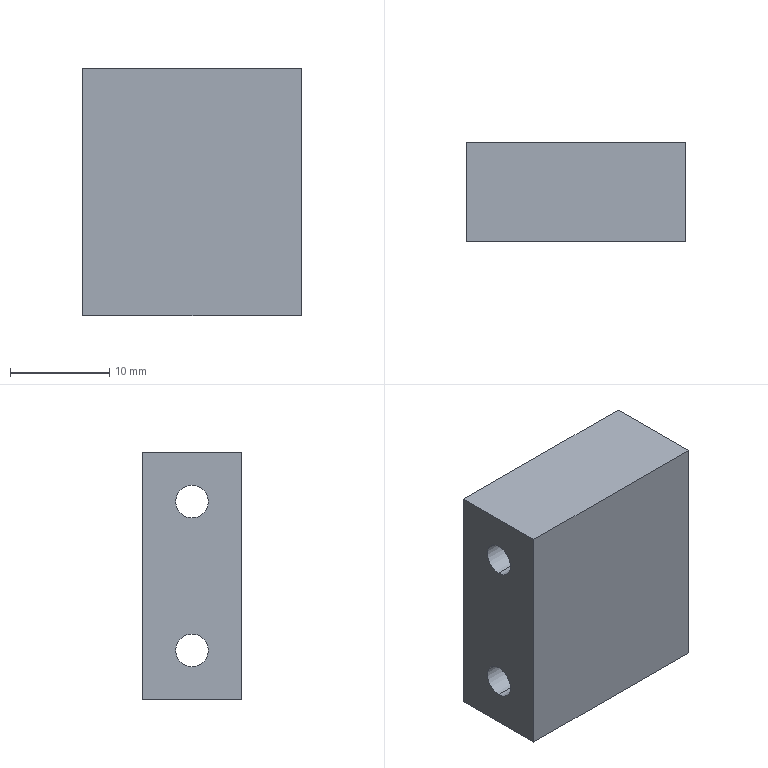Part | STEP file | 0246_220_Pin | 1 solid | 10 faces | box 22 x 10 x 25 mm | volume 5124 mm3 | plane 6 | cylinder 4 | commonest cylinder face diameters 3.3 x4
STEP:
#1=CARTESIAN_POINT('',(0.,0.,0.));
#2=DIRECTION('',(0.,0.,1.));
#3=DIRECTION('',(1.,0.,0.));
#4=AXIS2_PLACEMENT_3D('',#1,#2,#3);
#5=CARTESIAN_POINT('',(0.,5.,-5.85));
#6=VERTEX_POINT('',#5);
#7=CARTESIAN_POINT('',(-22.,5.,-5.85));
#8=VERTEX_POINT('',#7);
#9=CARTESIAN_POINT('',(-22.,5.,-5.85));
#10=DIRECTION('',(-1.,0.,0.));
#11=VECTOR('',#10,1.);
#12=LINE('',#9,#11);
#13=CARTESIAN_POINT('',(-22.,5.,-7.5));
#14=DIRECTION('',(-1.,0.,0.));
#15=DIRECTION('',(0.,0.,1.));
#16=AXIS2_PLACEMENT_3D('',#13,#14,#15);
#17=CYLINDRICAL_SURFACE('',#16,1.65);
#18=CARTESIAN_POINT('',(6.283,0.));
#19=DIRECTION('',(0.,1.));
#20=VECTOR('',#19,1.);
#21=LINE('',#18,#20);
#22=(GEOMETRIC_REPRESENTATION_CONTEXT(2)PARAMETRIC_REPRESENTATION_CONTEXT()REPRESENTATION_CONTEXT('',''));
#23=DEFINITIONAL_REPRESENTATION('',(#21),#22);
#24=PCURVE('',#17,#23);
#25=CARTESIAN_POINT('',(-22.,5.,-7.5));
#26=DIRECTION('',(-1.,0.,0.));
#27=DIRECTION('',(0.,0.,1.));
#28=AXIS2_PLACEMENT_3D('',#25,#26,#27);
#29=CYLINDRICAL_SURFACE('',#28,1.65);
#30=CARTESIAN_POINT('',(0.,0.));
#31=DIRECTION('',(0.,1.));
#32=VECTOR('',#31,1.);
#33=LINE('',#30,#32);
#34=(GEOMETRIC_REPRESENTATION_CONTEXT(2)PARAMETRIC_REPRESENTATION_CONTEXT()REPRESENTATION_CONTEXT('',''));
#35=DEFINITIONAL_REPRESENTATION('',(#33),#34);
#36=PCURVE('',#29,#35);
#37=SURFACE_CURVE('',#12,(#24,#36),.PCURVE_S1.);
#38=EDGE_CURVE('',#6,#8,#37,.T.);
#39=ORIENTED_EDGE('',*,*,#38,.T.);
#40=CARTESIAN_POINT('',(-22.,5.,-9.15));
#41=VERTEX_POINT('',#40);
#42=CARTESIAN_POINT('',(-22.,5.,-7.5));
#43=DIRECTION('',(-1.,0.,0.));
#44=DIRECTION('',(0.,0.,1.));
#45=AXIS2_PLACEMENT_3D('',#42,#43,#44);
#46=CIRCLE('',#45,1.65);
#47=CARTESIAN_POINT('',(0.,0.));
#48=DIRECTION('',(1.,0.));
#49=VECTOR('',#48,1.);
#50=LINE('',#47,#49);
#51=(GEOMETRIC_REPRESENTATION_CONTEXT(2)PARAMETRIC_REPRESENTATION_CONTEXT()REPRESENTATION_CONTEXT('',''));
#52=DEFINITIONAL_REPRESENTATION('',(#50),#51);
#53=PCURVE('',#17,#52);
#54=CARTESIAN_POINT('',(-22.,10.,-12.5));
#55=DIRECTION('',(1.,0.,0.));
#56=DIRECTION('',(0.,0.,-1.));
#57=AXIS2_PLACEMENT_3D('',#54,#55,#56);
#58=PLANE('',#57);
#59=CARTESIAN_POINT('',(-6.65,-5.));
#60=CARTESIAN_POINT('',(-6.65,-2.142));
#61=CARTESIAN_POINT('',(-4.175,-3.571));
#62=CARTESIAN_POINT('',(-1.7,-5.));
#63=CARTESIAN_POINT('',(-4.175,-6.429));
#64=CARTESIAN_POINT('',(-6.65,-7.858));
#65=CARTESIAN_POINT('',(-6.65,-5.));
#66=(BOUNDED_CURVE()B_SPLINE_CURVE(2,(#59,#60,#61,#62,#63,#64,#65),.UNSPECIFIED.,.T.,.F.)B_SPLINE_CURVE_WITH_KNOTS((1,2,2,2,2,1),(-2.094,0.,2.094,4.189,6.283,8.378),.UNSPECIFIED.)CURVE()GEOMETRIC_REPRESENTATION_ITEM()RATIONAL_B_SPLINE_CURVE((1.,0.5,1.,0.5,1.,0.5,1.))REPRESENTATION_ITEM(''));
#67=(GEOMETRIC_REPRESENTATION_CONTEXT(2)PARAMETRIC_REPRESENTATION_CONTEXT()REPRESENTATION_CONTEXT('',''));
#68=DEFINITIONAL_REPRESENTATION('',(#66),#67);
#69=PCURVE('',#58,#68);
#70=SURFACE_CURVE('',#46,(#53,#69),.PCURVE_S1.);
#71=EDGE_CURVE('',#41,#8,#70,.T.);
#72=ORIENTED_EDGE('',*,*,#71,.F.);
#73=CARTESIAN_POINT('',(0.,5.,-9.15));
#74=VERTEX_POINT('',#73);
#75=CARTESIAN_POINT('',(-22.,5.,-9.15));
#76=DIRECTION('',(-1.,0.,0.));
#77=VECTOR('',#76,1.);
#78=LINE('',#75,#77);
#79=CARTESIAN_POINT('',(3.142,0.));
#80=DIRECTION('',(0.,1.));
#81=VECTOR('',#80,1.);
#82=LINE('',#79,#81);
#83=(GEOMETRIC_REPRESENTATION_CONTEXT(2)PARAMETRIC_REPRESENTATION_CONTEXT()REPRESENTATION_CONTEXT('',''));
#84=DEFINITIONAL_REPRESENTATION('',(#82),#83);
#85=PCURVE('',#17,#84);
#86=CARTESIAN_POINT('',(3.142,0.));
#87=DIRECTION('',(0.,1.));
#88=VECTOR('',#87,1.);
#89=LINE('',#86,#88);
#90=(GEOMETRIC_REPRESENTATION_CONTEXT(2)PARAMETRIC_REPRESENTATION_CONTEXT()REPRESENTATION_CONTEXT('',''));
#91=DEFINITIONAL_REPRESENTATION('',(#89),#90);
#92=PCURVE('',#29,#91);
#93=SURFACE_CURVE('',#78,(#85,#92),.PCURVE_S1.);
#94=EDGE_CURVE('',#74,#41,#93,.T.);
#95=ORIENTED_EDGE('',*,*,#94,.F.);
#96=CARTESIAN_POINT('',(0.,5.,-7.5));
#97=DIRECTION('',(-1.,0.,0.));
#98=DIRECTION('',(0.,0.,1.));
#99=AXIS2_PLACEMENT_3D('',#96,#97,#98);
#100=CIRCLE('',#99,1.65);
#101=CARTESIAN_POINT('',(0.,-22.));
#102=DIRECTION('',(1.,0.));
#103=VECTOR('',#102,1.);
#104=LINE('',#101,#103);
#105=(GEOMETRIC_REPRESENTATION_CONTEXT(2)PARAMETRIC_REPRESENTATION_CONTEXT()REPRESENTATION_CONTEXT('',''));
#106=DEFINITIONAL_REPRESENTATION('',(#104),#105);
#107=PCURVE('',#17,#106);
#108=CARTESIAN_POINT('',(0.,10.,-12.5));
#109=DIRECTION('',(-1.,0.,0.));
#110=DIRECTION('',(0.,0.,1.));
#111=AXIS2_PLACEMENT_3D('',#108,#109,#110);
#112=PLANE('',#111);
#113=CARTESIAN_POINT('',(5.,-5.));
#114=DIRECTION('',(1.,0.));
#115=AXIS2_PLACEMENT_2D('',#113,#114);
#116=CIRCLE('',#115,1.65);
#117=(GEOMETRIC_REPRESENTATION_CONTEXT(2)PARAMETRIC_REPRESENTATION_CONTEXT()REPRESENTATION_CONTEXT('',''));
#118=DEFINITIONAL_REPRESENTATION('',(#116),#117);
#119=PCURVE('',#112,#118);
#120=SURFACE_CURVE('',#100,(#107,#119),.PCURVE_S1.);
#121=EDGE_CURVE('',#74,#6,#120,.T.);
#122=ORIENTED_EDGE('',*,*,#121,.T.);
#123=EDGE_LOOP('',(#39,#72,#95,#122));
#124=FACE_BOUND('',#123,.F.);
#125=ADVANCED_FACE('',(#124),#17,.F.);
#126=CARTESIAN_POINT('',(0.,5.,9.15));
#127=VERTEX_POINT('',#126);
#128=CARTESIAN_POINT('',(-22.,5.,9.15));
#129=VERTEX_POINT('',#128);
#130=CARTESIAN_POINT('',(-22.,5.,9.15));
#131=DIRECTION('',(-1.,0.,0.));
#132=VECTOR('',#131,1.);
#133=LINE('',#130,#132);
#134=CARTESIAN_POINT('',(-22.,5.,7.5));
#135=DIRECTION('',(-1.,0.,0.));
#136=DIRECTION('',(0.,0.,1.));
#137=AXIS2_PLACEMENT_3D('',#134,#135,#136);
#138=CYLINDRICAL_SURFACE('',#137,1.65);
#139=CARTESIAN_POINT('',(6.283,0.));
#140=DIRECTION('',(0.,1.));
#141=VECTOR('',#140,1.);
#142=LINE('',#139,#141);
#143=(GEOMETRIC_REPRESENTATION_CONTEXT(2)PARAMETRIC_REPRESENTATION_CONTEXT()REPRESENTATION_CONTEXT('',''));
#144=DEFINITIONAL_REPRESENTATION('',(#142),#143);
#145=PCURVE('',#138,#144);
#146=CARTESIAN_POINT('',(-22.,5.,7.5));
#147=DIRECTION('',(-1.,0.,0.));
#148=DIRECTION('',(0.,0.,1.));
#149=AXIS2_PLACEMENT_3D('',#146,#147,#148);
#150=CYLINDRICAL_SURFACE('',#149,1.65);
#151=CARTESIAN_POINT('',(0.,0.));
#152=DIRECTION('',(0.,1.));
#153=VECTOR('',#152,1.);
#154=LINE('',#151,#153);
#155=(GEOMETRIC_REPRESENTATION_CONTEXT(2)PARAMETRIC_REPRESENTATION_CONTEXT()REPRESENTATION_CONTEXT('',''));
#156=DEFINITIONAL_REPRESENTATION('',(#154),#155);
#157=PCURVE('',#150,#156);
#158=SURFACE_CURVE('',#133,(#145,#157),.PCURVE_S1.);
#159=EDGE_CURVE('',#127,#129,#158,.T.);
#160=ORIENTED_EDGE('',*,*,#159,.T.);
#161=CARTESIAN_POINT('',(-22.,5.,5.85));
#162=VERTEX_POINT('',#161);
#163=CARTESIAN_POINT('',(-22.,5.,7.5));
#164=DIRECTION('',(-1.,0.,0.));
#165=DIRECTION('',(0.,0.,1.));
#166=AXIS2_PLACEMENT_3D('',#163,#164,#165);
#167=CIRCLE('',#166,1.65);
#168=CARTESIAN_POINT('',(0.,0.));
#169=DIRECTION('',(1.,0.));
#170=VECTOR('',#169,1.);
#171=LINE('',#168,#170);
#172=(GEOMETRIC_REPRESENTATION_CONTEXT(2)PARAMETRIC_REPRESENTATION_CONTEXT()REPRESENTATION_CONTEXT('',''));
#173=DEFINITIONAL_REPRESENTATION('',(#171),#172);
#174=PCURVE('',#138,#173);
#175=CARTESIAN_POINT('',(-21.65,-5.));
#176=CARTESIAN_POINT('',(-21.65,-2.142));
#177=CARTESIAN_POINT('',(-19.175,-3.571));
#178=CARTESIAN_POINT('',(-16.7,-5.));
#179=CARTESIAN_POINT('',(-19.175,-6.429));
#180=CARTESIAN_POINT('',(-21.65,-7.858));
#181=CARTESIAN_POINT('',(-21.65,-5.));
#182=(BOUNDED_CURVE()B_SPLINE_CURVE(2,(#175,#176,#177,#178,#179,#180,#181),.UNSPECIFIED.,.T.,.F.)B_SPLINE_CURVE_WITH_KNOTS((1,2,2,2,2,1),(-2.094,0.,2.094,4.189,6.283,8.378),.UNSPECIFIED.)CURVE()GEOMETRIC_REPRESENTATION_ITEM()RATIONAL_B_SPLINE_CURVE((1.,0.5,1.,0.5,1.,0.5,1.))REPRESENTATION_ITEM(''));
#183=(GEOMETRIC_REPRESENTATION_CONTEXT(2)PARAMETRIC_REPRESENTATION_CONTEXT()REPRESENTATION_CONTEXT('',''));
#184=DEFINITIONAL_REPRESENTATION('',(#182),#183);
#185=PCURVE('',#58,#184);
#186=SURFACE_CURVE('',#167,(#174,#185),.PCURVE_S1.);
#187=EDGE_CURVE('',#162,#129,#186,.T.);
#188=ORIENTED_EDGE('',*,*,#187,.F.);
#189=CARTESIAN_POINT('',(0.,5.,5.85));
#190=VERTEX_POINT('',#189);
#191=CARTESIAN_POINT('',(-22.,5.,5.85));
#192=DIRECTION('',(-1.,0.,0.));
#193=VECTOR('',#192,1.);
#194=LINE('',#191,#193);
#195=CARTESIAN_POINT('',(3.142,0.));
#196=DIRECTION('',(0.,1.));
#197=VECTOR('',#196,1.);
#198=LINE('',#195,#197);
#199=(GEOMETRIC_REPRESENTATION_CONTEXT(2)PARAMETRIC_REPRESENTATION_CONTEXT()REPRESENTATION_CONTEXT('',''));
#200=DEFINITIONAL_REPRESENTATION('',(#198),#199);
#201=PCURVE('',#138,#200);
#202=CARTESIAN_POINT('',(3.142,0.));
#203=DIRECTION('',(0.,1.));
#204=VECTOR('',#203,1.);
#205=LINE('',#202,#204);
#206=(GEOMETRIC_REPRESENTATION_CONTEXT(2)PARAMETRIC_REPRESENTATION_CONTEXT()REPRESENTATION_CONTEXT('',''));
#207=DEFINITIONAL_REPRESENTATION('',(#205),#206);
#208=PCURVE('',#150,#207);
#209=SURFACE_CURVE('',#194,(#201,#208),.PCURVE_S1.);
#210=EDGE_CURVE('',#190,#162,#209,.T.);
#211=ORIENTED_EDGE('',*,*,#210,.F.);
#212=CARTESIAN_POINT('',(0.,5.,7.5));
#213=DIRECTION('',(-1.,0.,0.));
#214=DIRECTION('',(0.,0.,1.));
#215=AXIS2_PLACEMENT_3D('',#212,#213,#214);
#216=CIRCLE('',#215,1.65);
#217=CARTESIAN_POINT('',(0.,-22.));
#218=DIRECTION('',(1.,0.));
#219=VECTOR('',#218,1.);
#220=LINE('',#217,#219);
#221=(GEOMETRIC_REPRESENTATION_CONTEXT(2)PARAMETRIC_REPRESENTATION_CONTEXT()REPRESENTATION_CONTEXT('',''));
#222=DEFINITIONAL_REPRESENTATION('',(#220),#221);
#223=PCURVE('',#138,#222);
#224=CARTESIAN_POINT('',(20.,-5.));
#225=DIRECTION('',(1.,0.));
#226=AXIS2_PLACEMENT_2D('',#224,#225);
#227=CIRCLE('',#226,1.65);
#228=(GEOMETRIC_REPRESENTATION_CONTEXT(2)PARAMETRIC_REPRESENTATION_CONTEXT()REPRESENTATION_CONTEXT('',''));
#229=DEFINITIONAL_REPRESENTATION('',(#227),#228);
#230=PCURVE('',#112,#229);
#231=SURFACE_CURVE('',#216,(#223,#230),.PCURVE_S1.);
#232=EDGE_CURVE('',#190,#127,#231,.T.);
#233=ORIENTED_EDGE('',*,*,#232,.T.);
#234=EDGE_LOOP('',(#160,#188,#211,#233));
#235=FACE_BOUND('',#234,.F.);
#236=ADVANCED_FACE('',(#235),#138,.F.);
#237=CARTESIAN_POINT('',(-22.,5.,-7.5));
#238=DIRECTION('',(-1.,0.,0.));
#239=DIRECTION('',(0.,0.,1.));
#240=AXIS2_PLACEMENT_3D('',#237,#238,#239);
#241=CIRCLE('',#240,1.65);
#242=CARTESIAN_POINT('',(-6.65,-5.));
#243=CARTESIAN_POINT('',(-6.65,-2.142));
#244=CARTESIAN_POINT('',(-4.175,-3.571));
#245=CARTESIAN_POINT('',(-1.7,-5.));
#246=CARTESIAN_POINT('',(-4.175,-6.429));
#247=CARTESIAN_POINT('',(-6.65,-7.858));
#248=CARTESIAN_POINT('',(-6.65,-5.));
#249=(BOUNDED_CURVE()B_SPLINE_CURVE(2,(#242,#243,#244,#245,#246,#247,#248),.UNSPECIFIED.,.T.,.F.)B_SPLINE_CURVE_WITH_KNOTS((1,2,2,2,2,1),(-2.094,0.,2.094,4.189,6.283,8.378),.UNSPECIFIED.)CURVE()GEOMETRIC_REPRESENTATION_ITEM()RATIONAL_B_SPLINE_CURVE((1.,0.5,1.,0.5,1.,0.5,1.))REPRESENTATION_ITEM(''));
#250=(GEOMETRIC_REPRESENTATION_CONTEXT(2)PARAMETRIC_REPRESENTATION_CONTEXT()REPRESENTATION_CONTEXT('',''));
#251=DEFINITIONAL_REPRESENTATION('',(#249),#250);
#252=PCURVE('',#58,#251);
#253=CARTESIAN_POINT('',(0.,0.));
#254=DIRECTION('',(1.,0.));
#255=VECTOR('',#254,1.);
#256=LINE('',#253,#255);
#257=(GEOMETRIC_REPRESENTATION_CONTEXT(2)PARAMETRIC_REPRESENTATION_CONTEXT()REPRESENTATION_CONTEXT('',''));
#258=DEFINITIONAL_REPRESENTATION('',(#256),#257);
#259=PCURVE('',#29,#258);
#260=SURFACE_CURVE('',#241,(#252,#259),.PCURVE_S1.);
#261=EDGE_CURVE('',#8,#41,#260,.T.);
#262=ORIENTED_EDGE('',*,*,#261,.F.);
#263=ORIENTED_EDGE('',*,*,#71,.F.);
#264=EDGE_LOOP('',(#262,#263));
#265=FACE_BOUND('',#264,.T.);
#266=CARTESIAN_POINT('',(-22.,5.,7.5));
#267=DIRECTION('',(-1.,0.,0.));
#268=DIRECTION('',(0.,0.,1.));
#269=AXIS2_PLACEMENT_3D('',#266,#267,#268);
#270=CIRCLE('',#269,1.65);
#271=CARTESIAN_POINT('',(-21.65,-5.));
#272=CARTESIAN_POINT('',(-21.65,-2.142));
#273=CARTESIAN_POINT('',(-19.175,-3.571));
#274=CARTESIAN_POINT('',(-16.7,-5.));
#275=CARTESIAN_POINT('',(-19.175,-6.429));
#276=CARTESIAN_POINT('',(-21.65,-7.858));
#277=CARTESIAN_POINT('',(-21.65,-5.));
#278=(BOUNDED_CURVE()B_SPLINE_CURVE(2,(#271,#272,#273,#274,#275,#276,#277),.UNSPECIFIED.,.T.,.F.)B_SPLINE_CURVE_WITH_KNOTS((1,2,2,2,2,1),(-2.094,0.,2.094,4.189,6.283,8.378),.UNSPECIFIED.)CURVE()GEOMETRIC_REPRESENTATION_ITEM()RATIONAL_B_SPLINE_CURVE((1.,0.5,1.,0.5,1.,0.5,1.))REPRESENTATION_ITEM(''));
#279=(GEOMETRIC_REPRESENTATION_CONTEXT(2)PARAMETRIC_REPRESENTATION_CONTEXT()REPRESENTATION_CONTEXT('',''));
#280=DEFINITIONAL_REPRESENTATION('',(#278),#279);
#281=PCURVE('',#58,#280);
#282=CARTESIAN_POINT('',(0.,0.));
#283=DIRECTION('',(1.,0.));
#284=VECTOR('',#283,1.);
#285=LINE('',#282,#284);
#286=(GEOMETRIC_REPRESENTATION_CONTEXT(2)PARAMETRIC_REPRESENTATION_CONTEXT()REPRESENTATION_CONTEXT('',''));
#287=DEFINITIONAL_REPRESENTATION('',(#285),#286);
#288=PCURVE('',#150,#287);
#289=SURFACE_CURVE('',#270,(#281,#288),.PCURVE_S1.);
#290=EDGE_CURVE('',#129,#162,#289,.T.);
#291=ORIENTED_EDGE('',*,*,#290,.F.);
#292=ORIENTED_EDGE('',*,*,#187,.F.);
#293=EDGE_LOOP('',(#291,#292));
#294=FACE_BOUND('',#293,.T.);
#295=CARTESIAN_POINT('',(-22.,0.,-12.5));
#296=VERTEX_POINT('',#295);
#297=CARTESIAN_POINT('',(-22.,0.,12.5));
#298=VERTEX_POINT('',#297);
#299=CARTESIAN_POINT('',(-22.,0.,-12.5));
#300=DIRECTION('',(0.,0.,1.));
#301=VECTOR('',#300,1.);
#302=LINE('',#299,#301);
#303=CARTESIAN_POINT('',(0.,-10.));
#304=DIRECTION('',(-1.,0.));
#305=VECTOR('',#304,1.);
#306=LINE('',#303,#305);
#307=(GEOMETRIC_REPRESENTATION_CONTEXT(2)PARAMETRIC_REPRESENTATION_CONTEXT()REPRESENTATION_CONTEXT('',''));
#308=DEFINITIONAL_REPRESENTATION('',(#306),#307);
#309=PCURVE('',#58,#308);
#310=CARTESIAN_POINT('',(-22.,0.,12.5));
#311=DIRECTION('',(0.,1.,0.));
#312=DIRECTION('',(0.,0.,1.));
#313=AXIS2_PLACEMENT_3D('',#310,#311,#312);
#314=PLANE('',#313);
#315=CARTESIAN_POINT('',(-25.,0.));
#316=DIRECTION('',(1.,0.));
#317=VECTOR('',#316,1.);
#318=LINE('',#315,#317);
#319=(GEOMETRIC_REPRESENTATION_CONTEXT(2)PARAMETRIC_REPRESENTATION_CONTEXT()REPRESENTATION_CONTEXT('',''));
#320=DEFINITIONAL_REPRESENTATION('',(#318),#319);
#321=PCURVE('',#314,#320);
#322=SURFACE_CURVE('',#302,(#309,#321),.PCURVE_S1.);
#323=EDGE_CURVE('',#296,#298,#322,.T.);
#324=ORIENTED_EDGE('',*,*,#323,.T.);
#325=CARTESIAN_POINT('',(-22.,10.,12.5));
#326=VERTEX_POINT('',#325);
#327=CARTESIAN_POINT('',(-22.,10.,12.5));
#328=DIRECTION('',(0.,-1.,0.));
#329=VECTOR('',#328,1.);
#330=LINE('',#327,#329);
#331=CARTESIAN_POINT('',(-25.,0.));
#332=DIRECTION('',(0.,-1.));
#333=VECTOR('',#332,1.);
#334=LINE('',#331,#333);
#335=(GEOMETRIC_REPRESENTATION_CONTEXT(2)PARAMETRIC_REPRESENTATION_CONTEXT()REPRESENTATION_CONTEXT('',''));
#336=DEFINITIONAL_REPRESENTATION('',(#334),#335);
#337=PCURVE('',#58,#336);
#338=CARTESIAN_POINT('',(-22.,10.,12.5));
#339=DIRECTION('',(0.,0.,-1.));
#340=DIRECTION('',(-1.,0.,0.));
#341=AXIS2_PLACEMENT_3D('',#338,#339,#340);
#342=PLANE('',#341);
#343=CARTESIAN_POINT('',(0.,0.));
#344=DIRECTION('',(0.,-1.));
#345=VECTOR('',#344,1.);
#346=LINE('',#343,#345);
#347=(GEOMETRIC_REPRESENTATION_CONTEXT(2)PARAMETRIC_REPRESENTATION_CONTEXT()REPRESENTATION_CONTEXT('',''));
#348=DEFINITIONAL_REPRESENTATION('',(#346),#347);
#349=PCURVE('',#342,#348);
#350=SURFACE_CURVE('',#330,(#337,#349),.PCURVE_S1.);
#351=EDGE_CURVE('',#326,#298,#350,.T.);
#352=ORIENTED_EDGE('',*,*,#351,.F.);
#353=CARTESIAN_POINT('',(-22.,10.,-12.5));
#354=VERTEX_POINT('',#353);
#355=CARTESIAN_POINT('',(-22.,10.,-12.5));
#356=DIRECTION('',(0.,0.,1.));
#357=VECTOR('',#356,1.);
#358=LINE('',#355,#357);
#359=CARTESIAN_POINT('',(0.,0.));
#360=DIRECTION('',(-1.,0.));
#361=VECTOR('',#360,1.);
#362=LINE('',#359,#361);
#363=(GEOMETRIC_REPRESENTATION_CONTEXT(2)PARAMETRIC_REPRESENTATION_CONTEXT()REPRESENTATION_CONTEXT('',''));
#364=DEFINITIONAL_REPRESENTATION('',(#362),#363);
#365=PCURVE('',#58,#364);
#366=CARTESIAN_POINT('',(-22.,10.,12.5));
#367=DIRECTION('',(0.,1.,0.));
#368=DIRECTION('',(0.,0.,1.));
#369=AXIS2_PLACEMENT_3D('',#366,#367,#368);
#370=PLANE('',#369);
#371=CARTESIAN_POINT('',(-25.,0.));
#372=DIRECTION('',(1.,0.));
#373=VECTOR('',#372,1.);
#374=LINE('',#371,#373);
#375=(GEOMETRIC_REPRESENTATION_CONTEXT(2)PARAMETRIC_REPRESENTATION_CONTEXT()REPRESENTATION_CONTEXT('',''));
#376=DEFINITIONAL_REPRESENTATION('',(#374),#375);
#377=PCURVE('',#370,#376);
#378=SURFACE_CURVE('',#358,(#365,#377),.PCURVE_S1.);
#379=EDGE_CURVE('',#354,#326,#378,.T.);
#380=ORIENTED_EDGE('',*,*,#379,.F.);
#381=CARTESIAN_POINT('',(-22.,10.,-12.5));
#382=DIRECTION('',(0.,-1.,0.));
#383=VECTOR('',#382,1.);
#384=LINE('',#381,#383);
#385=CARTESIAN_POINT('',(0.,0.));
#386=DIRECTION('',(0.,-1.));
#387=VECTOR('',#386,1.);
#388=LINE('',#385,#387);
#389=(GEOMETRIC_REPRESENTATION_CONTEXT(2)PARAMETRIC_REPRESENTATION_CONTEXT()REPRESENTATION_CONTEXT('',''));
#390=DEFINITIONAL_REPRESENTATION('',(#388),#389);
#391=PCURVE('',#58,#390);
#392=CARTESIAN_POINT('',(-22.,10.,-12.5));
#393=DIRECTION('',(0.,0.,1.));
#394=DIRECTION('',(1.,0.,0.));
#395=AXIS2_PLACEMENT_3D('',#392,#393,#394);
#396=PLANE('',#395);
#397=CARTESIAN_POINT('',(0.,0.));
#398=DIRECTION('',(0.,-1.));
#399=VECTOR('',#398,1.);
#400=LINE('',#397,#399);
#401=(GEOMETRIC_REPRESENTATION_CONTEXT(2)PARAMETRIC_REPRESENTATION_CONTEXT()REPRESENTATION_CONTEXT('',''));
#402=DEFINITIONAL_REPRESENTATION('',(#400),#401);
#403=PCURVE('',#396,#402);
#404=SURFACE_CURVE('',#384,(#391,#403),.PCURVE_S1.);
#405=EDGE_CURVE('',#354,#296,#404,.T.);
#406=ORIENTED_EDGE('',*,*,#405,.T.);
#407=EDGE_LOOP('',(#324,#352,#380,#406));
#408=FACE_BOUND('',#407,.T.);
#409=ADVANCED_FACE('',(#265,#294,#408),#58,.F.);
#410=CARTESIAN_POINT('',(0.,0.,12.5));
#411=VERTEX_POINT('',#410);
#412=CARTESIAN_POINT('',(-22.,0.,12.5));
#413=DIRECTION('',(1.,0.,0.));
#414=VECTOR('',#413,1.);
#415=LINE('',#412,#414);
#416=CARTESIAN_POINT('',(0.,-10.));
#417=DIRECTION('',(-1.,0.));
#418=VECTOR('',#417,1.);
#419=LINE('',#416,#418);
#420=(GEOMETRIC_REPRESENTATION_CONTEXT(2)PARAMETRIC_REPRESENTATION_CONTEXT()REPRESENTATION_CONTEXT('',''));
#421=DEFINITIONAL_REPRESENTATION('',(#419),#420);
#422=PCURVE('',#342,#421);
#423=CARTESIAN_POINT('',(0.,0.));
#424=DIRECTION('',(0.,1.));
#425=VECTOR('',#424,1.);
#426=LINE('',#423,#425);
#427=(GEOMETRIC_REPRESENTATION_CONTEXT(2)PARAMETRIC_REPRESENTATION_CONTEXT()REPRESENTATION_CONTEXT('',''));
#428=DEFINITIONAL_REPRESENTATION('',(#426),#427);
#429=PCURVE('',#314,#428);
#430=SURFACE_CURVE('',#415,(#422,#429),.PCURVE_S1.);
#431=EDGE_CURVE('',#298,#411,#430,.T.);
#432=ORIENTED_EDGE('',*,*,#431,.T.);
#433=CARTESIAN_POINT('',(0.,10.,12.5));
#434=VERTEX_POINT('',#433);
#435=CARTESIAN_POINT('',(0.,10.,12.5));
#436=DIRECTION('',(0.,-1.,0.));
#437=VECTOR('',#436,1.);
#438=LINE('',#435,#437);
#439=CARTESIAN_POINT('',(-22.,0.));
#440=DIRECTION('',(0.,-1.));
#441=VECTOR('',#440,1.);
#442=LINE('',#439,#441);
#443=(GEOMETRIC_REPRESENTATION_CONTEXT(2)PARAMETRIC_REPRESENTATION_CONTEXT()REPRESENTATION_CONTEXT('',''));
#444=DEFINITIONAL_REPRESENTATION('',(#442),#443);
#445=PCURVE('',#342,#444);
#446=CARTESIAN_POINT('',(25.,0.));
#447=DIRECTION('',(0.,-1.));
#448=VECTOR('',#447,1.);
#449=LINE('',#446,#448);
#450=(GEOMETRIC_REPRESENTATION_CONTEXT(2)PARAMETRIC_REPRESENTATION_CONTEXT()REPRESENTATION_CONTEXT('',''));
#451=DEFINITIONAL_REPRESENTATION('',(#449),#450);
#452=PCURVE('',#112,#451);
#453=SURFACE_CURVE('',#438,(#445,#452),.PCURVE_S1.);
#454=EDGE_CURVE('',#434,#411,#453,.T.);
#455=ORIENTED_EDGE('',*,*,#454,.F.);
#456=CARTESIAN_POINT('',(-22.,10.,12.5));
#457=DIRECTION('',(1.,0.,0.));
#458=VECTOR('',#457,1.);
#459=LINE('',#456,#458);
#460=CARTESIAN_POINT('',(0.,0.));
#461=DIRECTION('',(-1.,0.));
#462=VECTOR('',#461,1.);
#463=LINE('',#460,#462);
#464=(GEOMETRIC_REPRESENTATION_CONTEXT(2)PARAMETRIC_REPRESENTATION_CONTEXT()REPRESENTATION_CONTEXT('',''));
#465=DEFINITIONAL_REPRESENTATION('',(#463),#464);
#466=PCURVE('',#342,#465);
#467=CARTESIAN_POINT('',(0.,0.));
#468=DIRECTION('',(0.,1.));
#469=VECTOR('',#468,1.);
#470=LINE('',#467,#469);
#471=(GEOMETRIC_REPRESENTATION_CONTEXT(2)PARAMETRIC_REPRESENTATION_CONTEXT()REPRESENTATION_CONTEXT('',''));
#472=DEFINITIONAL_REPRESENTATION('',(#470),#471);
#473=PCURVE('',#370,#472);
#474=SURFACE_CURVE('',#459,(#466,#473),.PCURVE_S1.);
#475=EDGE_CURVE('',#326,#434,#474,.T.);
#476=ORIENTED_EDGE('',*,*,#475,.F.);
#477=ORIENTED_EDGE('',*,*,#351,.T.);
#478=EDGE_LOOP('',(#432,#455,#476,#477));
#479=FACE_BOUND('',#478,.T.);
#480=ADVANCED_FACE('',(#479),#342,.F.);
#481=CARTESIAN_POINT('',(0.,5.,-7.5));
#482=DIRECTION('',(-1.,0.,0.));
#483=DIRECTION('',(0.,0.,1.));
#484=AXIS2_PLACEMENT_3D('',#481,#482,#483);
#485=CIRCLE('',#484,1.65);
#486=CARTESIAN_POINT('',(5.,-5.));
#487=DIRECTION('',(1.,0.));
#488=AXIS2_PLACEMENT_2D('',#486,#487);
#489=CIRCLE('',#488,1.65);
#490=(GEOMETRIC_REPRESENTATION_CONTEXT(2)PARAMETRIC_REPRESENTATION_CONTEXT()REPRESENTATION_CONTEXT('',''));
#491=DEFINITIONAL_REPRESENTATION('',(#489),#490);
#492=PCURVE('',#112,#491);
#493=CARTESIAN_POINT('',(0.,-22.));
#494=DIRECTION('',(1.,0.));
#495=VECTOR('',#494,1.);
#496=LINE('',#493,#495);
#497=(GEOMETRIC_REPRESENTATION_CONTEXT(2)PARAMETRIC_REPRESENTATION_CONTEXT()REPRESENTATION_CONTEXT('',''));
#498=DEFINITIONAL_REPRESENTATION('',(#496),#497);
#499=PCURVE('',#29,#498);
#500=SURFACE_CURVE('',#485,(#492,#499),.PCURVE_S1.);
#501=EDGE_CURVE('',#6,#74,#500,.T.);
#502=ORIENTED_EDGE('',*,*,#501,.T.);
#503=ORIENTED_EDGE('',*,*,#121,.T.);
#504=EDGE_LOOP('',(#502,#503));
#505=FACE_BOUND('',#504,.T.);
#506=CARTESIAN_POINT('',(0.,5.,7.5));
#507=DIRECTION('',(-1.,0.,0.));
#508=DIRECTION('',(0.,0.,1.));
#509=AXIS2_PLACEMENT_3D('',#506,#507,#508);
#510=CIRCLE('',#509,1.65);
#511=CARTESIAN_POINT('',(20.,-5.));
#512=DIRECTION('',(1.,0.));
#513=AXIS2_PLACEMENT_2D('',#511,#512);
#514=CIRCLE('',#513,1.65);
#515=(GEOMETRIC_REPRESENTATION_CONTEXT(2)PARAMETRIC_REPRESENTATION_CONTEXT()REPRESENTATION_CONTEXT('',''));
#516=DEFINITIONAL_REPRESENTATION('',(#514),#515);
#517=PCURVE('',#112,#516);
#518=CARTESIAN_POINT('',(0.,-22.));
#519=DIRECTION('',(1.,0.));
#520=VECTOR('',#519,1.);
#521=LINE('',#518,#520);
#522=(GEOMETRIC_REPRESENTATION_CONTEXT(2)PARAMETRIC_REPRESENTATION_CONTEXT()REPRESENTATION_CONTEXT('',''));
#523=DEFINITIONAL_REPRESENTATION('',(#521),#522);
#524=PCURVE('',#150,#523);
#525=SURFACE_CURVE('',#510,(#517,#524),.PCURVE_S1.);
#526=EDGE_CURVE('',#127,#190,#525,.T.);
#527=ORIENTED_EDGE('',*,*,#526,.T.);
#528=ORIENTED_EDGE('',*,*,#232,.T.);
#529=EDGE_LOOP('',(#527,#528));
#530=FACE_BOUND('',#529,.T.);
#531=CARTESIAN_POINT('',(0.,0.,-12.5));
#532=VERTEX_POINT('',#531);
#533=CARTESIAN_POINT('',(0.,0.,-12.5));
#534=DIRECTION('',(0.,0.,-1.));
#535=VECTOR('',#534,1.);
#536=LINE('',#533,#535);
#537=CARTESIAN_POINT('',(0.,-10.));
#538=DIRECTION('',(-1.,0.));
#539=VECTOR('',#538,1.);
#540=LINE('',#537,#539);
#541=(GEOMETRIC_REPRESENTATION_CONTEXT(2)PARAMETRIC_REPRESENTATION_CONTEXT()REPRESENTATION_CONTEXT('',''));
#542=DEFINITIONAL_REPRESENTATION('',(#540),#541);
#543=PCURVE('',#112,#542);
#544=CARTESIAN_POINT('',(-25.,22.));
#545=DIRECTION('',(-1.,0.));
#546=VECTOR('',#545,1.);
#547=LINE('',#544,#546);
#548=(GEOMETRIC_REPRESENTATION_CONTEXT(2)PARAMETRIC_REPRESENTATION_CONTEXT()REPRESENTATION_CONTEXT('',''));
#549=DEFINITIONAL_REPRESENTATION('',(#547),#548);
#550=PCURVE('',#314,#549);
#551=SURFACE_CURVE('',#536,(#543,#550),.PCURVE_S1.);
#552=EDGE_CURVE('',#411,#532,#551,.T.);
#553=ORIENTED_EDGE('',*,*,#552,.T.);
#554=CARTESIAN_POINT('',(0.,10.,-12.5));
#555=VERTEX_POINT('',#554);
#556=CARTESIAN_POINT('',(0.,10.,-12.5));
#557=DIRECTION('',(0.,-1.,0.));
#558=VECTOR('',#557,1.);
#559=LINE('',#556,#558);
#560=CARTESIAN_POINT('',(0.,0.));
#561=DIRECTION('',(0.,-1.));
#562=VECTOR('',#561,1.);
#563=LINE('',#560,#562);
#564=(GEOMETRIC_REPRESENTATION_CONTEXT(2)PARAMETRIC_REPRESENTATION_CONTEXT()REPRESENTATION_CONTEXT('',''));
#565=DEFINITIONAL_REPRESENTATION('',(#563),#564);
#566=PCURVE('',#112,#565);
#567=CARTESIAN_POINT('',(22.,0.));
#568=DIRECTION('',(0.,-1.));
#569=VECTOR('',#568,1.);
#570=LINE('',#567,#569);
#571=(GEOMETRIC_REPRESENTATION_CONTEXT(2)PARAMETRIC_REPRESENTATION_CONTEXT()REPRESENTATION_CONTEXT('',''));
#572=DEFINITIONAL_REPRESENTATION('',(#570),#571);
#573=PCURVE('',#396,#572);
#574=SURFACE_CURVE('',#559,(#566,#573),.PCURVE_S1.);
#575=EDGE_CURVE('',#555,#532,#574,.T.);
#576=ORIENTED_EDGE('',*,*,#575,.F.);
#577=CARTESIAN_POINT('',(0.,10.,-12.5));
#578=DIRECTION('',(0.,0.,-1.));
#579=VECTOR('',#578,1.);
#580=LINE('',#577,#579);
#581=CARTESIAN_POINT('',(0.,0.));
#582=DIRECTION('',(-1.,0.));
#583=VECTOR('',#582,1.);
#584=LINE('',#581,#583);
#585=(GEOMETRIC_REPRESENTATION_CONTEXT(2)PARAMETRIC_REPRESENTATION_CONTEXT()REPRESENTATION_CONTEXT('',''));
#586=DEFINITIONAL_REPRESENTATION('',(#584),#585);
#587=PCURVE('',#112,#586);
#588=CARTESIAN_POINT('',(-25.,22.));
#589=DIRECTION('',(-1.,0.));
#590=VECTOR('',#589,1.);
#591=LINE('',#588,#590);
#592=(GEOMETRIC_REPRESENTATION_CONTEXT(2)PARAMETRIC_REPRESENTATION_CONTEXT()REPRESENTATION_CONTEXT('',''));
#593=DEFINITIONAL_REPRESENTATION('',(#591),#592);
#594=PCURVE('',#370,#593);
#595=SURFACE_CURVE('',#580,(#587,#594),.PCURVE_S1.);
#596=EDGE_CURVE('',#434,#555,#595,.T.);
#597=ORIENTED_EDGE('',*,*,#596,.F.);
#598=ORIENTED_EDGE('',*,*,#454,.T.);
#599=EDGE_LOOP('',(#553,#576,#597,#598));
#600=FACE_BOUND('',#599,.T.);
#601=ADVANCED_FACE('',(#505,#530,#600),#112,.F.);
#602=CARTESIAN_POINT('',(-22.,0.,-12.5));
#603=DIRECTION('',(-1.,0.,0.));
#604=VECTOR('',#603,1.);
#605=LINE('',#602,#604);
#606=CARTESIAN_POINT('',(0.,-10.));
#607=DIRECTION('',(-1.,0.));
#608=VECTOR('',#607,1.);
#609=LINE('',#606,#608);
#610=(GEOMETRIC_REPRESENTATION_CONTEXT(2)PARAMETRIC_REPRESENTATION_CONTEXT()REPRESENTATION_CONTEXT('',''));
#611=DEFINITIONAL_REPRESENTATION('',(#609),#610);
#612=PCURVE('',#396,#611);
#613=CARTESIAN_POINT('',(-25.,0.));
#614=DIRECTION('',(0.,-1.));
#615=VECTOR('',#614,1.);
#616=LINE('',#613,#615);
#617=(GEOMETRIC_REPRESENTATION_CONTEXT(2)PARAMETRIC_REPRESENTATION_CONTEXT()REPRESENTATION_CONTEXT('',''));
#618=DEFINITIONAL_REPRESENTATION('',(#616),#617);
#619=PCURVE('',#314,#618);
#620=SURFACE_CURVE('',#605,(#612,#619),.PCURVE_S1.);
#621=EDGE_CURVE('',#532,#296,#620,.T.);
#622=ORIENTED_EDGE('',*,*,#621,.T.);
#623=ORIENTED_EDGE('',*,*,#405,.F.);
#624=CARTESIAN_POINT('',(-22.,10.,-12.5));
#625=DIRECTION('',(-1.,0.,0.));
#626=VECTOR('',#625,1.);
#627=LINE('',#624,#626);
#628=CARTESIAN_POINT('',(0.,0.));
#629=DIRECTION('',(-1.,0.));
#630=VECTOR('',#629,1.);
#631=LINE('',#628,#630);
#632=(GEOMETRIC_REPRESENTATION_CONTEXT(2)PARAMETRIC_REPRESENTATION_CONTEXT()REPRESENTATION_CONTEXT('',''));
#633=DEFINITIONAL_REPRESENTATION('',(#631),#632);
#634=PCURVE('',#396,#633);
#635=CARTESIAN_POINT('',(-25.,0.));
#636=DIRECTION('',(0.,-1.));
#637=VECTOR('',#636,1.);
#638=LINE('',#635,#637);
#639=(GEOMETRIC_REPRESENTATION_CONTEXT(2)PARAMETRIC_REPRESENTATION_CONTEXT()REPRESENTATION_CONTEXT('',''));
#640=DEFINITIONAL_REPRESENTATION('',(#638),#639);
#641=PCURVE('',#370,#640);
#642=SURFACE_CURVE('',#627,(#634,#641),.PCURVE_S1.);
#643=EDGE_CURVE('',#555,#354,#642,.T.);
#644=ORIENTED_EDGE('',*,*,#643,.F.);
#645=ORIENTED_EDGE('',*,*,#575,.T.);
#646=EDGE_LOOP('',(#622,#623,#644,#645));
#647=FACE_BOUND('',#646,.T.);
#648=ADVANCED_FACE('',(#647),#396,.F.);
#649=ORIENTED_EDGE('',*,*,#379,.T.);
#650=ORIENTED_EDGE('',*,*,#475,.T.);
#651=ORIENTED_EDGE('',*,*,#596,.T.);
#652=ORIENTED_EDGE('',*,*,#643,.T.);
#653=EDGE_LOOP('',(#649,#650,#651,#652));
#654=FACE_BOUND('',#653,.T.);
#655=ADVANCED_FACE('',(#654),#370,.T.);
#656=ORIENTED_EDGE('',*,*,#323,.F.);
#657=ORIENTED_EDGE('',*,*,#621,.F.);
#658=ORIENTED_EDGE('',*,*,#552,.F.);
#659=ORIENTED_EDGE('',*,*,#431,.F.);
#660=EDGE_LOOP('',(#656,#657,#658,#659));
#661=FACE_BOUND('',#660,.T.);
#662=ADVANCED_FACE('',(#661),#314,.F.);
#663=ORIENTED_EDGE('',*,*,#290,.F.);
#664=ORIENTED_EDGE('',*,*,#159,.F.);
#665=ORIENTED_EDGE('',*,*,#526,.T.);
#666=ORIENTED_EDGE('',*,*,#210,.T.);
#667=EDGE_LOOP('',(#663,#664,#665,#666));
#668=FACE_BOUND('',#667,.F.);
#669=ADVANCED_FACE('',(#668),#150,.F.);
#670=ORIENTED_EDGE('',*,*,#261,.F.);
#671=ORIENTED_EDGE('',*,*,#38,.F.);
#672=ORIENTED_EDGE('',*,*,#501,.T.);
#673=ORIENTED_EDGE('',*,*,#94,.T.);
#674=EDGE_LOOP('',(#670,#671,#672,#673));
#675=FACE_BOUND('',#674,.F.);
#676=ADVANCED_FACE('',(#675),#29,.F.);
#677=CLOSED_SHELL('',(#125,#236,#409,#480,#601,#648,#655,#662,#669,#676));
#678=MANIFOLD_SOLID_BREP('',#677);
#679=(LENGTH_UNIT()NAMED_UNIT(*)SI_UNIT(.MILLI.,.METRE.));
#680=UNCERTAINTY_MEASURE_WITH_UNIT(LENGTH_MEASURE(0.0000001),#679,'','');
#681=(NAMED_UNIT(*)PLANE_ANGLE_UNIT()SI_UNIT($,.RADIAN.));
#682=(NAMED_UNIT(*)SI_UNIT($,.STERADIAN.)SOLID_ANGLE_UNIT());
#683=(GEOMETRIC_REPRESENTATION_CONTEXT(3)GLOBAL_UNCERTAINTY_ASSIGNED_CONTEXT((#680))GLOBAL_UNIT_ASSIGNED_CONTEXT((#679,#681,#682))REPRESENTATION_CONTEXT('',''));
#684=ADVANCED_BREP_SHAPE_REPRESENTATION('',(#4,#678),#683);